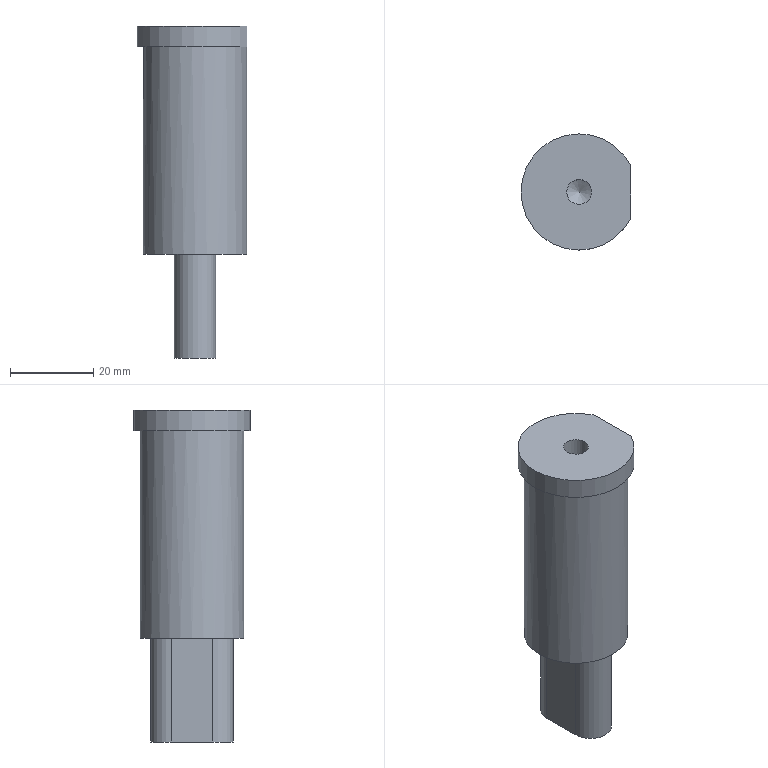Part | NX | features solid 2 | 1 solid | 13 faces | box 26.5 x 28 x 80 mm | volume 31638 mm3 | plane 7 | cylinder 5 | cone 1 | commonest cylinder face diameters 10 x2 6 x1 25 x1 28 x1
STEP:
#1=CARTESIAN_POINT('',(100.913,347.997,10.));
#2=VERTEX_POINT('',#1);
#3=CARTESIAN_POINT('',(113.413,347.997,10.));
#4=DIRECTION('',(0.,0.,-1.));
#5=DIRECTION('',(-1.,0.,0.));
#6=AXIS2_PLACEMENT_3D('',#3,#4,#5);
#7=CIRCLE('',#6,12.5);
#8=EDGE_CURVE('',#2,#2,#7,.T.);
#9=ORIENTED_EDGE('',*,*,#8,.T.);
#10=EDGE_LOOP('',(#9));
#11=FACE_BOUND('',#10,.T.);
#12=CARTESIAN_POINT('',(108.413,352.997,10.));
#13=VERTEX_POINT('',#12);
#14=CARTESIAN_POINT('',(108.413,342.997,10.));
#15=VERTEX_POINT('',#14);
#16=CARTESIAN_POINT('',(108.413,347.997,10.));
#17=DIRECTION('',(0.,-1.,0.));
#18=VECTOR('',#17,1000.);
#19=LINE('',#16,#18);
#20=EDGE_CURVE('',#13,#15,#19,.T.);
#21=ORIENTED_EDGE('',*,*,#20,.T.);
#22=CARTESIAN_POINT('',(118.413,342.997,10.));
#23=VERTEX_POINT('',#22);
#24=CARTESIAN_POINT('',(113.413,342.997,10.));
#25=DIRECTION('',(0.,0.,-1.));
#26=DIRECTION('',(-1.,0.,0.));
#27=AXIS2_PLACEMENT_3D('',#24,#25,#26);
#28=CIRCLE('',#27,5.);
#29=EDGE_CURVE('',#23,#15,#28,.T.);
#30=ORIENTED_EDGE('',*,*,#29,.F.);
#31=CARTESIAN_POINT('',(118.413,352.997,10.));
#32=VERTEX_POINT('',#31);
#33=CARTESIAN_POINT('',(118.413,347.997,10.));
#34=DIRECTION('',(0.,-1.,0.));
#35=VECTOR('',#34,1000.);
#36=LINE('',#33,#35);
#37=EDGE_CURVE('',#32,#23,#36,.T.);
#38=ORIENTED_EDGE('',*,*,#37,.F.);
#39=CARTESIAN_POINT('',(113.413,352.997,10.));
#40=DIRECTION('',(0.,0.,-1.));
#41=DIRECTION('',(-1.,0.,0.));
#42=AXIS2_PLACEMENT_3D('',#39,#40,#41);
#43=CIRCLE('',#42,5.);
#44=EDGE_CURVE('',#13,#32,#43,.T.);
#45=ORIENTED_EDGE('',*,*,#44,.F.);
#46=EDGE_LOOP('',(#21,#30,#38,#45));
#47=FACE_BOUND('',#46,.T.);
#48=CARTESIAN_POINT('',(113.413,347.997,10.));
#49=DIRECTION('',(0.,0.,1.));
#50=DIRECTION('',(-1.,0.,0.));
#51=AXIS2_PLACEMENT_3D('',#48,#49,#50);
#52=PLANE('',#51);
#53=ADVANCED_FACE('',(#11,#47),#52,.F.);
#54=ORIENTED_EDGE('',*,*,#8,.F.);
#55=EDGE_LOOP('',(#54));
#56=FACE_BOUND('',#55,.T.);
#57=CARTESIAN_POINT('',(125.913,347.997,60.));
#58=VERTEX_POINT('',#57);
#59=CARTESIAN_POINT('',(113.413,347.997,60.));
#60=DIRECTION('',(0.,0.,-1.));
#61=DIRECTION('',(-1.,0.,0.));
#62=AXIS2_PLACEMENT_3D('',#59,#60,#61);
#63=CIRCLE('',#62,12.5);
#64=EDGE_CURVE('',#58,#58,#63,.T.);
#65=ORIENTED_EDGE('',*,*,#64,.T.);
#66=EDGE_LOOP('',(#65));
#67=FACE_BOUND('',#66,.T.);
#68=CARTESIAN_POINT('',(113.413,347.997,65.));
#69=DIRECTION('',(0.,0.,-1.));
#70=DIRECTION('',(1.,0.,0.));
#71=AXIS2_PLACEMENT_3D('',#68,#69,#70);
#72=CYLINDRICAL_SURFACE('',#71,12.5);
#73=ADVANCED_FACE('',(#56,#67),#72,.T.);
#74=CARTESIAN_POINT('',(125.913,341.692,60.));
#75=VERTEX_POINT('',#74);
#76=CARTESIAN_POINT('',(125.913,354.301,60.));
#77=VERTEX_POINT('',#76);
#78=CARTESIAN_POINT('',(113.413,347.997,60.));
#79=DIRECTION('',(0.,0.,-1.));
#80=DIRECTION('',(-1.,0.,0.));
#81=AXIS2_PLACEMENT_3D('',#78,#79,#80);
#82=CIRCLE('',#81,14.);
#83=EDGE_CURVE('',#75,#77,#82,.T.);
#84=ORIENTED_EDGE('',*,*,#83,.T.);
#85=CARTESIAN_POINT('',(125.913,347.997,60.));
#86=DIRECTION('',(0.,1.,0.));
#87=VECTOR('',#86,1000.);
#88=LINE('',#85,#87);
#89=EDGE_CURVE('',#58,#77,#88,.T.);
#90=ORIENTED_EDGE('',*,*,#89,.F.);
#91=ORIENTED_EDGE('',*,*,#64,.F.);
#92=CARTESIAN_POINT('',(125.913,347.997,60.));
#93=DIRECTION('',(0.,1.,0.));
#94=VECTOR('',#93,1000.);
#95=LINE('',#92,#94);
#96=EDGE_CURVE('',#75,#58,#95,.T.);
#97=ORIENTED_EDGE('',*,*,#96,.F.);
#98=EDGE_LOOP('',(#84,#90,#91,#97));
#99=FACE_BOUND('',#98,.T.);
#100=CARTESIAN_POINT('',(113.413,347.997,60.));
#101=DIRECTION('',(0.,0.,1.));
#102=DIRECTION('',(-1.,0.,0.));
#103=AXIS2_PLACEMENT_3D('',#100,#101,#102);
#104=PLANE('',#103);
#105=ADVANCED_FACE('',(#99),#104,.F.);
#106=CARTESIAN_POINT('',(125.913,354.301,65.));
#107=VERTEX_POINT('',#106);
#108=CARTESIAN_POINT('',(125.913,354.301,70.));
#109=DIRECTION('',(0.,0.,-1.));
#110=VECTOR('',#109,1000.);
#111=LINE('',#108,#110);
#112=EDGE_CURVE('',#77,#107,#111,.F.);
#113=ORIENTED_EDGE('',*,*,#112,.F.);
#114=ORIENTED_EDGE('',*,*,#83,.F.);
#115=CARTESIAN_POINT('',(125.913,341.692,65.));
#116=VERTEX_POINT('',#115);
#117=CARTESIAN_POINT('',(125.913,341.692,70.));
#118=DIRECTION('',(0.,0.,-1.));
#119=VECTOR('',#118,1000.);
#120=LINE('',#117,#119);
#121=EDGE_CURVE('',#116,#75,#120,.T.);
#122=ORIENTED_EDGE('',*,*,#121,.F.);
#123=CARTESIAN_POINT('',(113.413,347.997,65.));
#124=DIRECTION('',(0.,0.,-1.));
#125=DIRECTION('',(-1.,0.,0.));
#126=AXIS2_PLACEMENT_3D('',#123,#124,#125);
#127=CIRCLE('',#126,14.);
#128=EDGE_CURVE('',#116,#107,#127,.T.);
#129=ORIENTED_EDGE('',*,*,#128,.T.);
#130=EDGE_LOOP('',(#113,#114,#122,#129));
#131=FACE_BOUND('',#130,.T.);
#132=CARTESIAN_POINT('',(113.413,347.997,60.));
#133=DIRECTION('',(0.,0.,1.));
#134=DIRECTION('',(-1.,0.,0.));
#135=AXIS2_PLACEMENT_3D('',#132,#133,#134);
#136=CYLINDRICAL_SURFACE('',#135,14.);
#137=ADVANCED_FACE('',(#131),#136,.T.);
#138=CARTESIAN_POINT('',(116.413,347.997,65.));
#139=VERTEX_POINT('',#138);
#140=CARTESIAN_POINT('',(113.413,347.997,65.));
#141=DIRECTION('',(0.,0.,1.));
#142=DIRECTION('',(1.,0.,0.));
#143=AXIS2_PLACEMENT_3D('',#140,#141,#142);
#144=CIRCLE('',#143,3.);
#145=EDGE_CURVE('',#139,#139,#144,.T.);
#146=ORIENTED_EDGE('',*,*,#145,.F.);
#147=EDGE_LOOP('',(#146));
#148=FACE_BOUND('',#147,.T.);
#149=CARTESIAN_POINT('',(125.913,347.997,65.));
#150=DIRECTION('',(0.,1.,0.));
#151=VECTOR('',#150,1000.);
#152=LINE('',#149,#151);
#153=EDGE_CURVE('',#116,#107,#152,.T.);
#154=ORIENTED_EDGE('',*,*,#153,.T.);
#155=ORIENTED_EDGE('',*,*,#128,.F.);
#156=EDGE_LOOP('',(#154,#155));
#157=FACE_BOUND('',#156,.T.);
#158=CARTESIAN_POINT('',(113.413,347.997,65.));
#159=DIRECTION('',(0.,0.,1.));
#160=DIRECTION('',(-1.,0.,0.));
#161=AXIS2_PLACEMENT_3D('',#158,#159,#160);
#162=PLANE('',#161);
#163=ADVANCED_FACE('',(#148,#157),#162,.T.);
#164=ORIENTED_EDGE('',*,*,#121,.T.);
#165=ORIENTED_EDGE('',*,*,#96,.T.);
#166=ORIENTED_EDGE('',*,*,#89,.T.);
#167=ORIENTED_EDGE('',*,*,#112,.T.);
#168=ORIENTED_EDGE('',*,*,#153,.F.);
#169=EDGE_LOOP('',(#164,#165,#166,#167,#168));
#170=FACE_BOUND('',#169,.T.);
#171=CARTESIAN_POINT('',(125.913,354.301,70.));
#172=DIRECTION('',(-1.,0.,0.));
#173=DIRECTION('',(0.,0.,-1.));
#174=AXIS2_PLACEMENT_3D('',#171,#172,#173);
#175=PLANE('',#174);
#176=ADVANCED_FACE('',(#170),#175,.F.);
#177=CARTESIAN_POINT('',(108.413,352.997,-15.));
#178=VERTEX_POINT('',#177);
#179=CARTESIAN_POINT('',(108.413,352.997,-15.));
#180=DIRECTION('',(0.,0.,1.));
#181=VECTOR('',#180,1000.);
#182=LINE('',#179,#181);
#183=EDGE_CURVE('',#178,#13,#182,.T.);
#184=ORIENTED_EDGE('',*,*,#183,.F.);
#185=CARTESIAN_POINT('',(108.413,342.997,-15.));
#186=VERTEX_POINT('',#185);
#187=CARTESIAN_POINT('',(108.413,352.997,-15.));
#188=DIRECTION('',(0.,-1.,0.));
#189=VECTOR('',#188,1000.);
#190=LINE('',#187,#189);
#191=EDGE_CURVE('',#178,#186,#190,.T.);
#192=ORIENTED_EDGE('',*,*,#191,.T.);
#193=CARTESIAN_POINT('',(108.413,342.997,-15.));
#194=DIRECTION('',(0.,0.,1.));
#195=VECTOR('',#194,1000.);
#196=LINE('',#193,#195);
#197=EDGE_CURVE('',#186,#15,#196,.T.);
#198=ORIENTED_EDGE('',*,*,#197,.T.);
#199=ORIENTED_EDGE('',*,*,#20,.F.);
#200=EDGE_LOOP('',(#184,#192,#198,#199));
#201=FACE_BOUND('',#200,.T.);
#202=CARTESIAN_POINT('',(108.413,352.997,-15.));
#203=DIRECTION('',(1.,0.,0.));
#204=DIRECTION('',(0.,0.,1.));
#205=AXIS2_PLACEMENT_3D('',#202,#203,#204);
#206=PLANE('',#205);
#207=ADVANCED_FACE('',(#201),#206,.F.);
#208=ORIENTED_EDGE('',*,*,#29,.T.);
#209=ORIENTED_EDGE('',*,*,#197,.F.);
#210=CARTESIAN_POINT('',(118.413,342.997,-15.));
#211=VERTEX_POINT('',#210);
#212=CARTESIAN_POINT('',(113.413,342.997,-15.));
#213=DIRECTION('',(0.,0.,-1.));
#214=DIRECTION('',(-1.,0.,0.));
#215=AXIS2_PLACEMENT_3D('',#212,#213,#214);
#216=CIRCLE('',#215,5.);
#217=EDGE_CURVE('',#211,#186,#216,.T.);
#218=ORIENTED_EDGE('',*,*,#217,.F.);
#219=CARTESIAN_POINT('',(118.413,342.997,-15.));
#220=DIRECTION('',(0.,0.,1.));
#221=VECTOR('',#220,1000.);
#222=LINE('',#219,#221);
#223=EDGE_CURVE('',#211,#23,#222,.T.);
#224=ORIENTED_EDGE('',*,*,#223,.T.);
#225=EDGE_LOOP('',(#208,#209,#218,#224));
#226=FACE_BOUND('',#225,.T.);
#227=CARTESIAN_POINT('',(113.413,342.997,-15.));
#228=DIRECTION('',(0.,0.,1.));
#229=DIRECTION('',(-1.,0.,0.));
#230=AXIS2_PLACEMENT_3D('',#227,#228,#229);
#231=CYLINDRICAL_SURFACE('',#230,5.);
#232=ADVANCED_FACE('',(#226),#231,.T.);
#233=ORIENTED_EDGE('',*,*,#37,.T.);
#234=ORIENTED_EDGE('',*,*,#223,.F.);
#235=CARTESIAN_POINT('',(118.413,352.997,-15.));
#236=VERTEX_POINT('',#235);
#237=CARTESIAN_POINT('',(118.413,352.997,-15.));
#238=DIRECTION('',(0.,-1.,0.));
#239=VECTOR('',#238,1000.);
#240=LINE('',#237,#239);
#241=EDGE_CURVE('',#236,#211,#240,.T.);
#242=ORIENTED_EDGE('',*,*,#241,.F.);
#243=CARTESIAN_POINT('',(118.413,352.997,-15.));
#244=DIRECTION('',(0.,0.,1.));
#245=VECTOR('',#244,1000.);
#246=LINE('',#243,#245);
#247=EDGE_CURVE('',#236,#32,#246,.T.);
#248=ORIENTED_EDGE('',*,*,#247,.T.);
#249=EDGE_LOOP('',(#233,#234,#242,#248));
#250=FACE_BOUND('',#249,.T.);
#251=CARTESIAN_POINT('',(118.413,352.997,-15.));
#252=DIRECTION('',(1.,0.,0.));
#253=DIRECTION('',(0.,0.,1.));
#254=AXIS2_PLACEMENT_3D('',#251,#252,#253);
#255=PLANE('',#254);
#256=ADVANCED_FACE('',(#250),#255,.T.);
#257=ORIENTED_EDGE('',*,*,#44,.T.);
#258=ORIENTED_EDGE('',*,*,#247,.F.);
#259=CARTESIAN_POINT('',(113.413,352.997,-15.));
#260=DIRECTION('',(0.,0.,-1.));
#261=DIRECTION('',(-1.,0.,0.));
#262=AXIS2_PLACEMENT_3D('',#259,#260,#261);
#263=CIRCLE('',#262,5.);
#264=EDGE_CURVE('',#178,#236,#263,.T.);
#265=ORIENTED_EDGE('',*,*,#264,.F.);
#266=ORIENTED_EDGE('',*,*,#183,.T.);
#267=EDGE_LOOP('',(#257,#258,#265,#266));
#268=FACE_BOUND('',#267,.T.);
#269=CARTESIAN_POINT('',(113.413,352.997,-15.));
#270=DIRECTION('',(0.,0.,1.));
#271=DIRECTION('',(-1.,0.,0.));
#272=AXIS2_PLACEMENT_3D('',#269,#270,#271);
#273=CYLINDRICAL_SURFACE('',#272,5.);
#274=ADVANCED_FACE('',(#268),#273,.T.);
#275=ORIENTED_EDGE('',*,*,#191,.F.);
#276=ORIENTED_EDGE('',*,*,#264,.T.);
#277=ORIENTED_EDGE('',*,*,#241,.T.);
#278=ORIENTED_EDGE('',*,*,#217,.T.);
#279=EDGE_LOOP('',(#275,#276,#277,#278));
#280=FACE_BOUND('',#279,.T.);
#281=CARTESIAN_POINT('',(113.413,342.997,-15.));
#282=DIRECTION('',(0.,0.,1.));
#283=DIRECTION('',(-1.,0.,0.));
#284=AXIS2_PLACEMENT_3D('',#281,#282,#283);
#285=PLANE('',#284);
#286=ADVANCED_FACE('',(#280),#285,.F.);
#287=CARTESIAN_POINT('',(116.413,347.997,52.));
#288=VERTEX_POINT('',#287);
#289=CARTESIAN_POINT('',(113.413,347.997,52.));
#290=DIRECTION('',(0.,0.,1.));
#291=DIRECTION('',(1.,0.,0.));
#292=AXIS2_PLACEMENT_3D('',#289,#290,#291);
#293=CIRCLE('',#292,3.);
#294=EDGE_CURVE('',#288,#288,#293,.T.);
#295=ORIENTED_EDGE('',*,*,#294,.T.);
#296=EDGE_LOOP('',(#295));
#297=FACE_BOUND('',#296,.T.);
#298=CARTESIAN_POINT('',(113.413,347.997,50.268));
#299=VERTEX_POINT('',#298);
#300=VERTEX_LOOP('',#299);
#301=FACE_BOUND('',#300,.T.);
#302=CARTESIAN_POINT('',(113.413,347.997,52.));
#303=DIRECTION('',(0.,0.,1.));
#304=DIRECTION('',(-1.,0.,0.));
#305=AXIS2_PLACEMENT_3D('',#302,#303,#304);
#306=CONICAL_SURFACE('',#305,3.,1.047);
#307=ADVANCED_FACE('',(#297,#301),#306,.F.);
#308=ORIENTED_EDGE('',*,*,#294,.F.);
#309=EDGE_LOOP('',(#308));
#310=FACE_BOUND('',#309,.T.);
#311=ORIENTED_EDGE('',*,*,#145,.T.);
#312=EDGE_LOOP('',(#311));
#313=FACE_BOUND('',#312,.T.);
#314=CARTESIAN_POINT('',(113.413,347.997,65.));
#315=DIRECTION('',(0.,0.,-1.));
#316=DIRECTION('',(1.,0.,0.));
#317=AXIS2_PLACEMENT_3D('',#314,#315,#316);
#318=CYLINDRICAL_SURFACE('',#317,3.);
#319=ADVANCED_FACE('',(#310,#313),#318,.F.);
#320=CLOSED_SHELL('',(#53,#73,#105,#137,#163,#176,#207,#232,#256,#274,#286,#307,#319));
#321=MANIFOLD_SOLID_BREP('',#320);
#322=(LENGTH_UNIT()NAMED_UNIT(*)SI_UNIT(.MILLI.,.METRE.));
#323=UNCERTAINTY_MEASURE_WITH_UNIT(LENGTH_MEASURE(0.00001),#322,'','');
#324=(NAMED_UNIT(*)PLANE_ANGLE_UNIT()SI_UNIT($,.RADIAN.));
#325=(NAMED_UNIT(*)SI_UNIT($,.STERADIAN.)SOLID_ANGLE_UNIT());
#326=(GEOMETRIC_REPRESENTATION_CONTEXT(3)GLOBAL_UNCERTAINTY_ASSIGNED_CONTEXT((#323))GLOBAL_UNIT_ASSIGNED_CONTEXT((#322,#324,#325))REPRESENTATION_CONTEXT('',''));
#327=ADVANCED_BREP_SHAPE_REPRESENTATION('',(#321),#326);